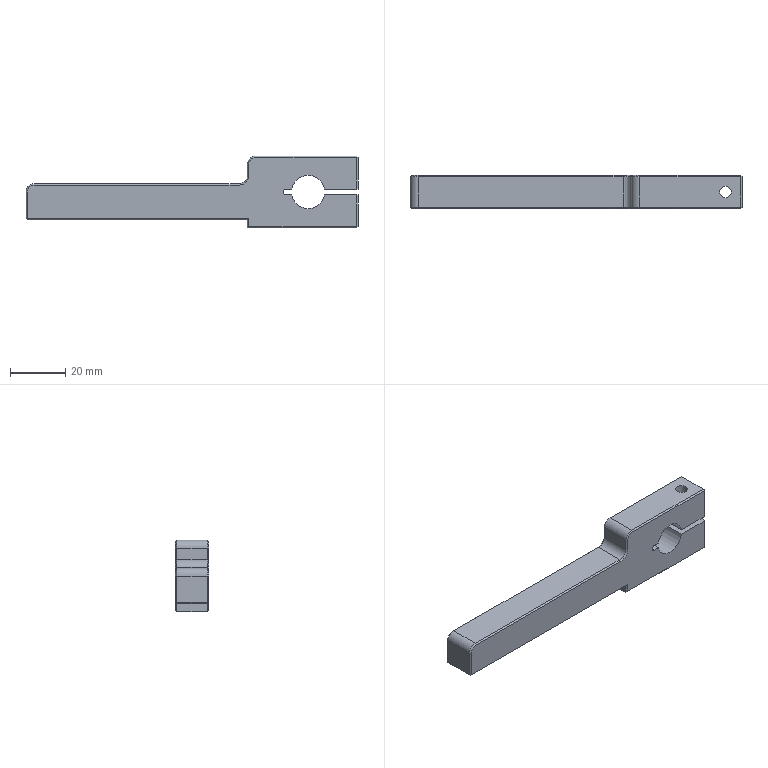Part | STEP file | ND25021-01-JDKM-50-TL | 1 solid | 68 faces | box 120 x 12 x 26 mm | volume 22518 mm3 | plane 42 | cylinder 16 | cone 10 | commonest cylinder face diameters 3.3 x4 6 x3 12 x3 2 x2 4.2 x2 5.5 x2